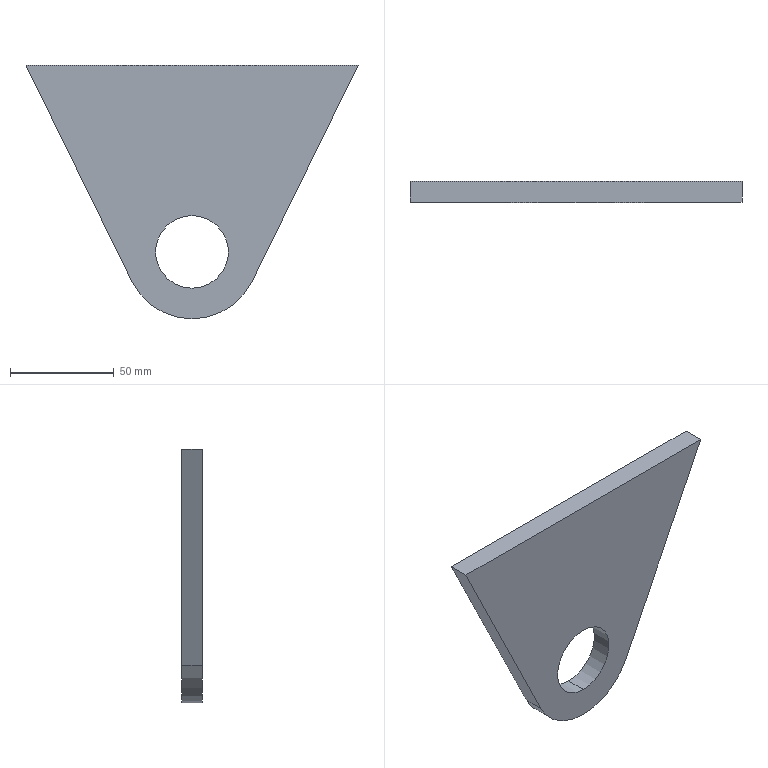Part | SolidWorks | features Extrusion 1, ICE 1 | 1 solid | 9 faces | box 160 x 10 x 122.25 mm | volume 111394 mm3 | plane 5 | cylinder 4 | commonest cylinder face diameters 35 x2 64.5 x2
STEP:
#1=CARTESIAN_POINT('',(80.,0.,-107.5));
#2=VERTEX_POINT('',#1);
#3=CARTESIAN_POINT('',(80.,0.,-72.5));
#4=VERTEX_POINT('',#3);
#5=CARTESIAN_POINT('',(80.,0.,-90.));
#6=DIRECTION('',(0.,1.,0.));
#7=DIRECTION('',(0.,0.,1.));
#8=AXIS2_PLACEMENT_3D('',#5,#6,#7);
#9=CIRCLE('',#8,17.5);
#10=EDGE_CURVE('',#2,#4,#9,.T.);
#11=ORIENTED_EDGE('',*,*,#10,.F.);
#12=CARTESIAN_POINT('',(80.,10.,-107.5));
#13=VERTEX_POINT('',#12);
#14=CARTESIAN_POINT('',(80.,0.,-107.5));
#15=DIRECTION('',(0.,1.,0.));
#16=VECTOR('',#15,1000.);
#17=LINE('',#14,#16);
#18=EDGE_CURVE('',#2,#13,#17,.T.);
#19=ORIENTED_EDGE('',*,*,#18,.T.);
#20=CARTESIAN_POINT('',(80.,10.,-72.5));
#21=VERTEX_POINT('',#20);
#22=CARTESIAN_POINT('',(80.,10.,-90.));
#23=DIRECTION('',(0.,1.,0.));
#24=DIRECTION('',(0.,0.,1.));
#25=AXIS2_PLACEMENT_3D('',#22,#23,#24);
#26=CIRCLE('',#25,17.5);
#27=EDGE_CURVE('',#13,#21,#26,.T.);
#28=ORIENTED_EDGE('',*,*,#27,.T.);
#29=CARTESIAN_POINT('',(80.,0.,-72.5));
#30=DIRECTION('',(0.,1.,0.));
#31=VECTOR('',#30,1000.);
#32=LINE('',#29,#31);
#33=EDGE_CURVE('',#4,#21,#32,.T.);
#34=ORIENTED_EDGE('',*,*,#33,.F.);
#35=EDGE_LOOP('',(#11,#19,#28,#34));
#36=FACE_OUTER_BOUND('',#35,.T.);
#37=CARTESIAN_POINT('',(80.,0.,-90.));
#38=DIRECTION('',(0.,1.,0.));
#39=DIRECTION('',(0.,0.,1.));
#40=AXIS2_PLACEMENT_3D('',#37,#38,#39);
#41=CYLINDRICAL_SURFACE('',#40,17.5);
#42=ADVANCED_FACE('',(#36),#41,.F.);
#43=CARTESIAN_POINT('',(80.,10.,-122.25));
#44=VERTEX_POINT('',#43);
#45=CARTESIAN_POINT('',(51.038,10.,-104.187));
#46=VERTEX_POINT('',#45);
#47=CARTESIAN_POINT('',(80.,10.,-90.));
#48=DIRECTION('',(0.,1.,0.));
#49=DIRECTION('',(0.,0.,1.));
#50=AXIS2_PLACEMENT_3D('',#47,#48,#49);
#51=CIRCLE('',#50,32.25);
#52=EDGE_CURVE('',#44,#46,#51,.T.);
#53=ORIENTED_EDGE('',*,*,#52,.F.);
#54=CARTESIAN_POINT('',(80.,0.,-122.25));
#55=VERTEX_POINT('',#54);
#56=CARTESIAN_POINT('',(80.,10.,-122.25));
#57=DIRECTION('',(0.,-1.,0.));
#58=VECTOR('',#57,1000.);
#59=LINE('',#56,#58);
#60=EDGE_CURVE('',#44,#55,#59,.T.);
#61=ORIENTED_EDGE('',*,*,#60,.T.);
#62=CARTESIAN_POINT('',(51.038,0.,-104.187));
#63=VERTEX_POINT('',#62);
#64=CARTESIAN_POINT('',(80.,0.,-90.));
#65=DIRECTION('',(0.,1.,0.));
#66=DIRECTION('',(0.,0.,1.));
#67=AXIS2_PLACEMENT_3D('',#64,#65,#66);
#68=CIRCLE('',#67,32.25);
#69=EDGE_CURVE('',#55,#63,#68,.T.);
#70=ORIENTED_EDGE('',*,*,#69,.T.);
#71=CARTESIAN_POINT('',(51.038,10.,-104.187));
#72=DIRECTION('',(0.,-1.,0.));
#73=VECTOR('',#72,1000.);
#74=LINE('',#71,#73);
#75=EDGE_CURVE('',#46,#63,#74,.T.);
#76=ORIENTED_EDGE('',*,*,#75,.F.);
#77=EDGE_LOOP('',(#53,#61,#70,#76));
#78=FACE_OUTER_BOUND('',#77,.T.);
#79=CARTESIAN_POINT('',(80.,10.,-90.));
#80=DIRECTION('',(0.,-1.,0.));
#81=DIRECTION('',(0.,0.,-1.));
#82=AXIS2_PLACEMENT_3D('',#79,#80,#81);
#83=CYLINDRICAL_SURFACE('',#82,32.25);
#84=ADVANCED_FACE('',(#78),#83,.T.);
#85=CARTESIAN_POINT('',(80.,10.,-90.));
#86=DIRECTION('',(0.,1.,0.));
#87=DIRECTION('',(0.,0.,1.));
#88=AXIS2_PLACEMENT_3D('',#85,#86,#87);
#89=CIRCLE('',#88,17.5);
#90=EDGE_CURVE('',#21,#13,#89,.T.);
#91=ORIENTED_EDGE('',*,*,#90,.F.);
#92=ORIENTED_EDGE('',*,*,#27,.F.);
#93=EDGE_LOOP('',(#91,#92));
#94=FACE_BOUND('',#93,.T.);
#95=CARTESIAN_POINT('',(0.,10.,0.));
#96=VERTEX_POINT('',#95);
#97=CARTESIAN_POINT('',(0.,10.,0.));
#98=DIRECTION('',(-0.4399,0.,0.898));
#99=VECTOR('',#98,1000.);
#100=LINE('',#97,#99);
#101=EDGE_CURVE('',#46,#96,#100,.T.);
#102=ORIENTED_EDGE('',*,*,#101,.T.);
#103=CARTESIAN_POINT('',(160.,10.,0.));
#104=VERTEX_POINT('',#103);
#105=CARTESIAN_POINT('',(0.,10.,0.));
#106=DIRECTION('',(1.,0.,0.));
#107=VECTOR('',#106,1000.);
#108=LINE('',#105,#107);
#109=EDGE_CURVE('',#96,#104,#108,.T.);
#110=ORIENTED_EDGE('',*,*,#109,.T.);
#111=CARTESIAN_POINT('',(108.962,10.,-104.187));
#112=VERTEX_POINT('',#111);
#113=CARTESIAN_POINT('',(160.,10.,0.));
#114=DIRECTION('',(-0.4399,0.,-0.898));
#115=VECTOR('',#114,1000.);
#116=LINE('',#113,#115);
#117=EDGE_CURVE('',#104,#112,#116,.T.);
#118=ORIENTED_EDGE('',*,*,#117,.T.);
#119=CARTESIAN_POINT('',(80.,10.,-90.));
#120=DIRECTION('',(0.,1.,0.));
#121=DIRECTION('',(0.,0.,1.));
#122=AXIS2_PLACEMENT_3D('',#119,#120,#121);
#123=CIRCLE('',#122,32.25);
#124=EDGE_CURVE('',#112,#44,#123,.T.);
#125=ORIENTED_EDGE('',*,*,#124,.T.);
#126=ORIENTED_EDGE('',*,*,#52,.T.);
#127=EDGE_LOOP('',(#102,#110,#118,#125,#126));
#128=FACE_OUTER_BOUND('',#127,.T.);
#129=CARTESIAN_POINT('',(80.,10.,-90.));
#130=DIRECTION('',(0.,1.,0.));
#131=DIRECTION('',(0.,0.,1.));
#132=AXIS2_PLACEMENT_3D('',#129,#130,#131);
#133=PLANE('',#132);
#134=ADVANCED_FACE('',(#94,#128),#133,.T.);
#135=CARTESIAN_POINT('',(80.,0.,-90.));
#136=DIRECTION('',(0.,1.,0.));
#137=DIRECTION('',(0.,0.,1.));
#138=AXIS2_PLACEMENT_3D('',#135,#136,#137);
#139=CIRCLE('',#138,17.5);
#140=EDGE_CURVE('',#4,#2,#139,.T.);
#141=ORIENTED_EDGE('',*,*,#140,.T.);
#142=ORIENTED_EDGE('',*,*,#10,.T.);
#143=EDGE_LOOP('',(#141,#142));
#144=FACE_BOUND('',#143,.T.);
#145=CARTESIAN_POINT('',(0.,0.,0.));
#146=VERTEX_POINT('',#145);
#147=CARTESIAN_POINT('',(0.,0.,0.));
#148=DIRECTION('',(-0.4399,0.,0.898));
#149=VECTOR('',#148,1000.);
#150=LINE('',#147,#149);
#151=EDGE_CURVE('',#63,#146,#150,.T.);
#152=ORIENTED_EDGE('',*,*,#151,.F.);
#153=ORIENTED_EDGE('',*,*,#69,.F.);
#154=CARTESIAN_POINT('',(108.962,0.,-104.187));
#155=VERTEX_POINT('',#154);
#156=CARTESIAN_POINT('',(80.,0.,-90.));
#157=DIRECTION('',(0.,1.,0.));
#158=DIRECTION('',(0.,0.,1.));
#159=AXIS2_PLACEMENT_3D('',#156,#157,#158);
#160=CIRCLE('',#159,32.25);
#161=EDGE_CURVE('',#155,#55,#160,.T.);
#162=ORIENTED_EDGE('',*,*,#161,.F.);
#163=CARTESIAN_POINT('',(160.,0.,0.));
#164=VERTEX_POINT('',#163);
#165=CARTESIAN_POINT('',(160.,0.,0.));
#166=DIRECTION('',(-0.4399,0.,-0.898));
#167=VECTOR('',#166,1000.);
#168=LINE('',#165,#167);
#169=EDGE_CURVE('',#164,#155,#168,.T.);
#170=ORIENTED_EDGE('',*,*,#169,.F.);
#171=CARTESIAN_POINT('',(0.,0.,0.));
#172=DIRECTION('',(1.,0.,0.));
#173=VECTOR('',#172,1000.);
#174=LINE('',#171,#173);
#175=EDGE_CURVE('',#146,#164,#174,.T.);
#176=ORIENTED_EDGE('',*,*,#175,.F.);
#177=EDGE_LOOP('',(#152,#153,#162,#170,#176));
#178=FACE_OUTER_BOUND('',#177,.T.);
#179=CARTESIAN_POINT('',(80.,0.,-90.));
#180=DIRECTION('',(0.,1.,0.));
#181=DIRECTION('',(0.,0.,1.));
#182=AXIS2_PLACEMENT_3D('',#179,#180,#181);
#183=PLANE('',#182);
#184=ADVANCED_FACE('',(#144,#178),#183,.F.);
#185=ORIENTED_EDGE('',*,*,#151,.T.);
#186=CARTESIAN_POINT('',(0.,10.,0.));
#187=DIRECTION('',(0.,-1.,0.));
#188=VECTOR('',#187,1000.);
#189=LINE('',#186,#188);
#190=EDGE_CURVE('',#96,#146,#189,.T.);
#191=ORIENTED_EDGE('',*,*,#190,.F.);
#192=ORIENTED_EDGE('',*,*,#101,.F.);
#193=ORIENTED_EDGE('',*,*,#75,.T.);
#194=EDGE_LOOP('',(#185,#191,#192,#193));
#195=FACE_OUTER_BOUND('',#194,.T.);
#196=CARTESIAN_POINT('',(0.,10.,0.));
#197=DIRECTION('',(0.898,0.,0.4399));
#198=DIRECTION('',(0.4399,0.,-0.898));
#199=AXIS2_PLACEMENT_3D('',#196,#197,#198);
#200=PLANE('',#199);
#201=ADVANCED_FACE('',(#195),#200,.F.);
#202=ORIENTED_EDGE('',*,*,#175,.T.);
#203=CARTESIAN_POINT('',(160.,10.,0.));
#204=DIRECTION('',(0.,-1.,0.));
#205=VECTOR('',#204,1000.);
#206=LINE('',#203,#205);
#207=EDGE_CURVE('',#104,#164,#206,.T.);
#208=ORIENTED_EDGE('',*,*,#207,.F.);
#209=ORIENTED_EDGE('',*,*,#109,.F.);
#210=ORIENTED_EDGE('',*,*,#190,.T.);
#211=EDGE_LOOP('',(#202,#208,#209,#210));
#212=FACE_OUTER_BOUND('',#211,.T.);
#213=CARTESIAN_POINT('',(0.,10.,0.));
#214=DIRECTION('',(0.,0.,-1.));
#215=DIRECTION('',(-1.,0.,0.));
#216=AXIS2_PLACEMENT_3D('',#213,#214,#215);
#217=PLANE('',#216);
#218=ADVANCED_FACE('',(#212),#217,.F.);
#219=ORIENTED_EDGE('',*,*,#169,.T.);
#220=CARTESIAN_POINT('',(108.962,10.,-104.187));
#221=DIRECTION('',(0.,-1.,0.));
#222=VECTOR('',#221,1000.);
#223=LINE('',#220,#222);
#224=EDGE_CURVE('',#112,#155,#223,.T.);
#225=ORIENTED_EDGE('',*,*,#224,.F.);
#226=ORIENTED_EDGE('',*,*,#117,.F.);
#227=ORIENTED_EDGE('',*,*,#207,.T.);
#228=EDGE_LOOP('',(#219,#225,#226,#227));
#229=FACE_OUTER_BOUND('',#228,.T.);
#230=CARTESIAN_POINT('',(160.,10.,0.));
#231=DIRECTION('',(-0.898,0.,0.4399));
#232=DIRECTION('',(0.4399,0.,0.898));
#233=AXIS2_PLACEMENT_3D('',#230,#231,#232);
#234=PLANE('',#233);
#235=ADVANCED_FACE('',(#229),#234,.F.);
#236=ORIENTED_EDGE('',*,*,#60,.F.);
#237=ORIENTED_EDGE('',*,*,#124,.F.);
#238=ORIENTED_EDGE('',*,*,#224,.T.);
#239=ORIENTED_EDGE('',*,*,#161,.T.);
#240=EDGE_LOOP('',(#236,#237,#238,#239));
#241=FACE_OUTER_BOUND('',#240,.T.);
#242=CARTESIAN_POINT('',(80.,10.,-90.));
#243=DIRECTION('',(0.,-1.,0.));
#244=DIRECTION('',(0.,0.,-1.));
#245=AXIS2_PLACEMENT_3D('',#242,#243,#244);
#246=CYLINDRICAL_SURFACE('',#245,32.25);
#247=ADVANCED_FACE('',(#241),#246,.T.);
#248=ORIENTED_EDGE('',*,*,#18,.F.);
#249=ORIENTED_EDGE('',*,*,#140,.F.);
#250=ORIENTED_EDGE('',*,*,#33,.T.);
#251=ORIENTED_EDGE('',*,*,#90,.T.);
#252=EDGE_LOOP('',(#248,#249,#250,#251));
#253=FACE_OUTER_BOUND('',#252,.T.);
#254=CARTESIAN_POINT('',(80.,0.,-90.));
#255=DIRECTION('',(0.,1.,0.));
#256=DIRECTION('',(0.,0.,1.));
#257=AXIS2_PLACEMENT_3D('',#254,#255,#256);
#258=CYLINDRICAL_SURFACE('',#257,17.5);
#259=ADVANCED_FACE('',(#253),#258,.F.);
#260=CLOSED_SHELL('',(#42,#84,#134,#184,#201,#218,#235,#247,#259));
#261=MANIFOLD_SOLID_BREP('',#260);
#262=CARTESIAN_POINT('',(0.,0.,0.));
#263=DIRECTION('',(0.,0.,1.));
#264=DIRECTION('',(1.,0.,0.));
#265=AXIS2_PLACEMENT_3D('',#262,#263,#264);
#266=(LENGTH_UNIT()NAMED_UNIT(*)SI_UNIT(.MILLI.,.METRE.));
#267=UNCERTAINTY_MEASURE_WITH_UNIT(LENGTH_MEASURE(0.00001),#266,'','');
#268=(NAMED_UNIT(*)PLANE_ANGLE_UNIT()SI_UNIT($,.RADIAN.));
#269=(NAMED_UNIT(*)SI_UNIT($,.STERADIAN.)SOLID_ANGLE_UNIT());
#270=(GEOMETRIC_REPRESENTATION_CONTEXT(3)GLOBAL_UNCERTAINTY_ASSIGNED_CONTEXT((#267))GLOBAL_UNIT_ASSIGNED_CONTEXT((#266,#268,#269))REPRESENTATION_CONTEXT('',''));
#271=ADVANCED_BREP_SHAPE_REPRESENTATION('',(#261,#265),#270);